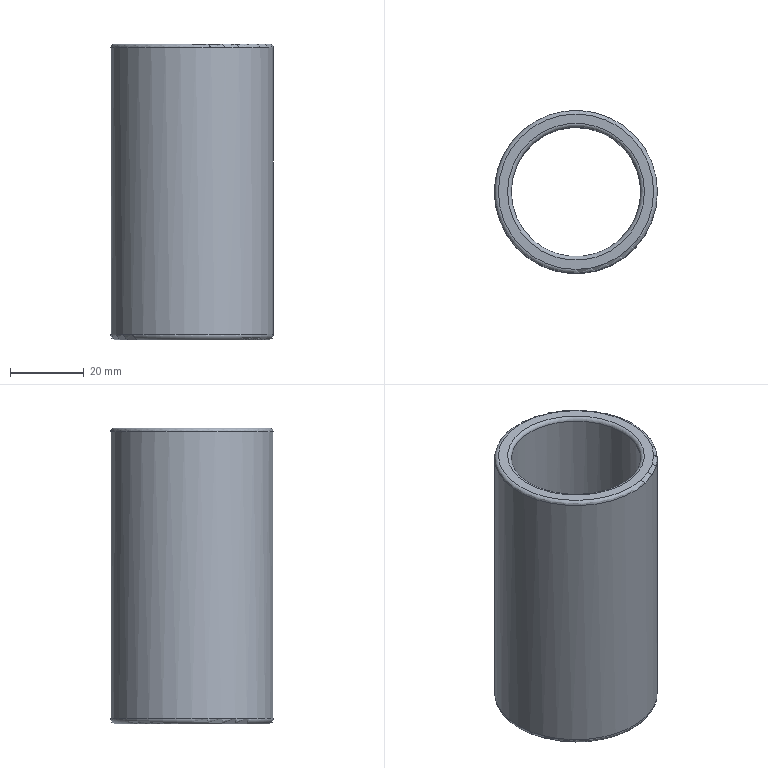Part | STEP file | 200 mesh_id50_xmt | 1 solid | 8 faces | box 44 x 44 x 80 mm | volume 44500 mm3 | torus 4 | plane 2 | cylinder 2 | commonest cylinder face diameters 35 x1 44 x1
STEP:
#1=CARTESIAN_POINT('',(-17071.884,-4158.269,96.));
#2=VERTEX_POINT('',#1);
#3=CARTESIAN_POINT('',(-17052.884,-4158.269,96.));
#4=DIRECTION('',(0.,0.,1.));
#5=DIRECTION('',(-1.,0.,0.));
#6=AXIS2_PLACEMENT_3D('',#3,#4,#5);
#7=CIRCLE('',#6,19.);
#8=EDGE_CURVE('',#2,#2,#7,.T.);
#9=ORIENTED_EDGE('',*,*,#8,.T.);
#10=EDGE_LOOP('',(#9));
#11=FACE_BOUND('',#10,.T.);
#12=CARTESIAN_POINT('',(-17073.384,-4158.269,96.));
#13=VERTEX_POINT('',#12);
#14=CARTESIAN_POINT('',(-17052.884,-4158.269,96.));
#15=DIRECTION('',(0.,0.,-1.));
#16=DIRECTION('',(-1.,0.,0.));
#17=AXIS2_PLACEMENT_3D('',#14,#15,#16);
#18=CIRCLE('',#17,20.5);
#19=EDGE_CURVE('',#13,#13,#18,.T.);
#20=ORIENTED_EDGE('',*,*,#19,.T.);
#21=EDGE_LOOP('',(#20));
#22=FACE_BOUND('',#21,.T.);
#23=CARTESIAN_POINT('',(-17052.884,-4158.269,96.));
#24=DIRECTION('',(0.,0.,-1.));
#25=DIRECTION('',(-1.,0.,0.));
#26=AXIS2_PLACEMENT_3D('',#23,#24,#25);
#27=PLANE('',#26);
#28=ADVANCED_FACE('',(#11,#22),#27,.T.);
#29=CARTESIAN_POINT('',(-17031.884,-4158.269,176.));
#30=VERTEX_POINT('',#29);
#31=CARTESIAN_POINT('',(-17052.884,-4158.269,176.));
#32=DIRECTION('',(0.,0.,1.));
#33=DIRECTION('',(1.,0.,0.));
#34=AXIS2_PLACEMENT_3D('',#31,#32,#33);
#35=CIRCLE('',#34,21.);
#36=EDGE_CURVE('',#30,#30,#35,.T.);
#37=ORIENTED_EDGE('',*,*,#36,.T.);
#38=EDGE_LOOP('',(#37));
#39=FACE_BOUND('',#38,.T.);
#40=CARTESIAN_POINT('',(-17034.384,-4158.269,176.));
#41=VERTEX_POINT('',#40);
#42=CARTESIAN_POINT('',(-17052.884,-4158.269,176.));
#43=DIRECTION('',(0.,0.,-1.));
#44=DIRECTION('',(1.,0.,0.));
#45=AXIS2_PLACEMENT_3D('',#42,#43,#44);
#46=CIRCLE('',#45,18.5);
#47=EDGE_CURVE('',#41,#41,#46,.T.);
#48=ORIENTED_EDGE('',*,*,#47,.T.);
#49=EDGE_LOOP('',(#48));
#50=FACE_BOUND('',#49,.T.);
#51=CARTESIAN_POINT('',(-17052.884,-4158.269,176.));
#52=DIRECTION('',(0.,0.,1.));
#53=DIRECTION('',(1.,0.,0.));
#54=AXIS2_PLACEMENT_3D('',#51,#52,#53);
#55=PLANE('',#54);
#56=ADVANCED_FACE('',(#39,#50),#55,.T.);
#57=CARTESIAN_POINT('',(-17030.884,-4158.269,175.));
#58=VERTEX_POINT('',#57);
#59=CARTESIAN_POINT('',(-17052.884,-4158.269,175.));
#60=DIRECTION('',(0.,0.,-1.));
#61=DIRECTION('',(1.,0.,0.));
#62=AXIS2_PLACEMENT_3D('',#59,#60,#61);
#63=CIRCLE('',#62,22.);
#64=EDGE_CURVE('',#58,#58,#63,.T.);
#65=ORIENTED_EDGE('',*,*,#64,.T.);
#66=EDGE_LOOP('',(#65));
#67=FACE_BOUND('',#66,.T.);
#68=CARTESIAN_POINT('',(-17074.884,-4158.269,97.5));
#69=VERTEX_POINT('',#68);
#70=CARTESIAN_POINT('',(-17052.884,-4158.269,97.5));
#71=DIRECTION('',(0.,0.,1.));
#72=DIRECTION('',(-1.,0.,0.));
#73=AXIS2_PLACEMENT_3D('',#70,#71,#72);
#74=CIRCLE('',#73,22.);
#75=EDGE_CURVE('',#69,#69,#74,.T.);
#76=ORIENTED_EDGE('',*,*,#75,.T.);
#77=EDGE_LOOP('',(#76));
#78=FACE_BOUND('',#77,.T.);
#79=CARTESIAN_POINT('',(-17052.884,-4158.269,176.));
#80=DIRECTION('',(0.,0.,-1.));
#81=DIRECTION('',(1.,0.,0.));
#82=AXIS2_PLACEMENT_3D('',#79,#80,#81);
#83=CYLINDRICAL_SURFACE('',#82,22.);
#84=ADVANCED_FACE('',(#67,#78),#83,.T.);
#85=CARTESIAN_POINT('',(-17035.384,-4158.269,175.));
#86=VERTEX_POINT('',#85);
#87=CARTESIAN_POINT('',(-17052.884,-4158.269,175.));
#88=DIRECTION('',(0.,0.,1.));
#89=DIRECTION('',(1.,0.,0.));
#90=AXIS2_PLACEMENT_3D('',#87,#88,#89);
#91=CIRCLE('',#90,17.5);
#92=EDGE_CURVE('',#86,#86,#91,.T.);
#93=ORIENTED_EDGE('',*,*,#92,.T.);
#94=EDGE_LOOP('',(#93));
#95=FACE_BOUND('',#94,.T.);
#96=CARTESIAN_POINT('',(-17070.384,-4158.269,97.5));
#97=VERTEX_POINT('',#96);
#98=CARTESIAN_POINT('',(-17052.884,-4158.269,97.5));
#99=DIRECTION('',(0.,0.,-1.));
#100=DIRECTION('',(-1.,0.,0.));
#101=AXIS2_PLACEMENT_3D('',#98,#99,#100);
#102=CIRCLE('',#101,17.5);
#103=EDGE_CURVE('',#97,#97,#102,.T.);
#104=ORIENTED_EDGE('',*,*,#103,.T.);
#105=EDGE_LOOP('',(#104));
#106=FACE_BOUND('',#105,.T.);
#107=CARTESIAN_POINT('',(-17052.884,-4158.269,176.));
#108=DIRECTION('',(0.,0.,-1.));
#109=DIRECTION('',(-1.,0.,0.));
#110=AXIS2_PLACEMENT_3D('',#107,#108,#109);
#111=CYLINDRICAL_SURFACE('',#110,17.5);
#112=ADVANCED_FACE('',(#95,#106),#111,.F.);
#113=ORIENTED_EDGE('',*,*,#8,.F.);
#114=EDGE_LOOP('',(#113));
#115=FACE_BOUND('',#114,.T.);
#116=ORIENTED_EDGE('',*,*,#103,.F.);
#117=EDGE_LOOP('',(#116));
#118=FACE_BOUND('',#117,.T.);
#119=CARTESIAN_POINT('',(-17052.884,-4158.269,97.5));
#120=DIRECTION('',(0.,0.,-1.));
#121=DIRECTION('',(-1.,0.,0.));
#122=AXIS2_PLACEMENT_3D('',#119,#120,#121);
#123=TOROIDAL_SURFACE('',#122,19.,1.5);
#124=ADVANCED_FACE('',(#115,#118),#123,.T.);
#125=ORIENTED_EDGE('',*,*,#19,.F.);
#126=EDGE_LOOP('',(#125));
#127=FACE_BOUND('',#126,.T.);
#128=ORIENTED_EDGE('',*,*,#75,.F.);
#129=EDGE_LOOP('',(#128));
#130=FACE_BOUND('',#129,.T.);
#131=CARTESIAN_POINT('',(-17052.884,-4158.269,97.5));
#132=DIRECTION('',(0.,0.,-1.));
#133=DIRECTION('',(-1.,0.,0.));
#134=AXIS2_PLACEMENT_3D('',#131,#132,#133);
#135=TOROIDAL_SURFACE('',#134,20.5,1.5);
#136=ADVANCED_FACE('',(#127,#130),#135,.T.);
#137=ORIENTED_EDGE('',*,*,#36,.F.);
#138=EDGE_LOOP('',(#137));
#139=FACE_BOUND('',#138,.T.);
#140=ORIENTED_EDGE('',*,*,#64,.F.);
#141=EDGE_LOOP('',(#140));
#142=FACE_BOUND('',#141,.T.);
#143=CARTESIAN_POINT('',(-17052.884,-4158.269,175.));
#144=DIRECTION('',(0.,0.,1.));
#145=DIRECTION('',(1.,0.,0.));
#146=AXIS2_PLACEMENT_3D('',#143,#144,#145);
#147=TOROIDAL_SURFACE('',#146,21.,1.);
#148=ADVANCED_FACE('',(#139,#142),#147,.T.);
#149=ORIENTED_EDGE('',*,*,#92,.F.);
#150=EDGE_LOOP('',(#149));
#151=FACE_BOUND('',#150,.T.);
#152=ORIENTED_EDGE('',*,*,#47,.F.);
#153=EDGE_LOOP('',(#152));
#154=FACE_BOUND('',#153,.T.);
#155=CARTESIAN_POINT('',(-17052.884,-4158.269,175.));
#156=DIRECTION('',(0.,0.,1.));
#157=DIRECTION('',(1.,0.,0.));
#158=AXIS2_PLACEMENT_3D('',#155,#156,#157);
#159=TOROIDAL_SURFACE('',#158,18.5,1.);
#160=ADVANCED_FACE('',(#151,#154),#159,.T.);
#161=CLOSED_SHELL('',(#28,#56,#84,#112,#124,#136,#148,#160));
#162=MANIFOLD_SOLID_BREP('',#161);
#163=(LENGTH_UNIT()NAMED_UNIT(*)SI_UNIT(.MILLI.,.METRE.));
#164=UNCERTAINTY_MEASURE_WITH_UNIT(LENGTH_MEASURE(0.00002),#163,'','');
#165=(NAMED_UNIT(*)PLANE_ANGLE_UNIT()SI_UNIT($,.RADIAN.));
#166=PLANE_ANGLE_MEASURE_WITH_UNIT(PLANE_ANGLE_MEASURE(0.01745),#165);
#167=DIMENSIONAL_EXPONENTS(0.,0.,0.,0.,0.,0.,0.);
#168=(CONVERSION_BASED_UNIT('DEGREE',#166)NAMED_UNIT(#167)PLANE_ANGLE_UNIT());
#169=(NAMED_UNIT(*)SI_UNIT($,.STERADIAN.)SOLID_ANGLE_UNIT());
#170=(GEOMETRIC_REPRESENTATION_CONTEXT(3)GLOBAL_UNCERTAINTY_ASSIGNED_CONTEXT((#164))GLOBAL_UNIT_ASSIGNED_CONTEXT((#163,#168,#169))REPRESENTATION_CONTEXT('',''));
#171=ADVANCED_BREP_SHAPE_REPRESENTATION('',(#162),#170);